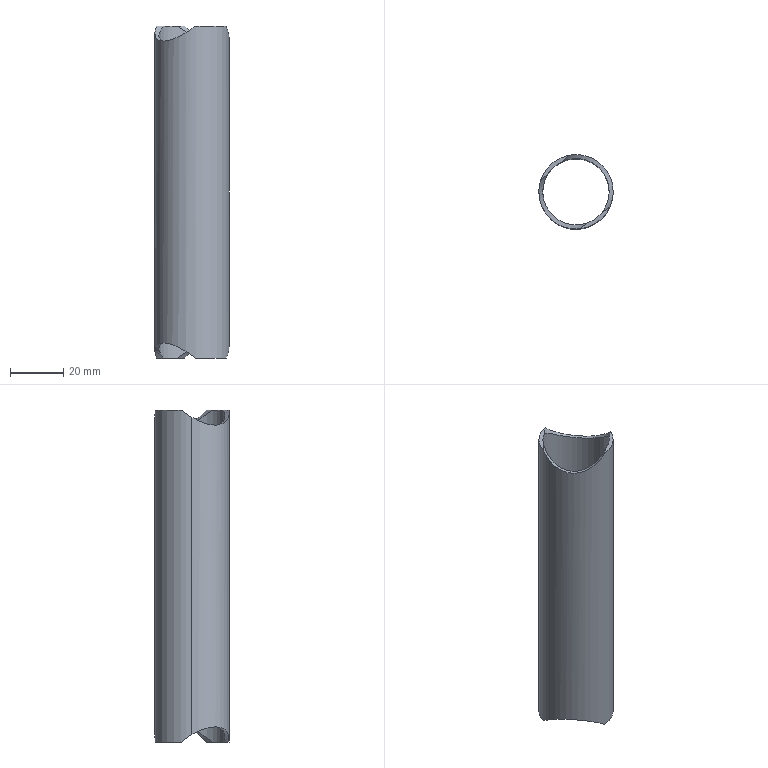Part | STEP file | PRT0001_68_7 | 1 solid | 12 faces | box 28.01 x 28.01 x 125 mm | volume 14806 mm3 | cylinder 8 | plane 4 | commonest cylinder face diameters 28 x4 25.01 x2 28.01 x2